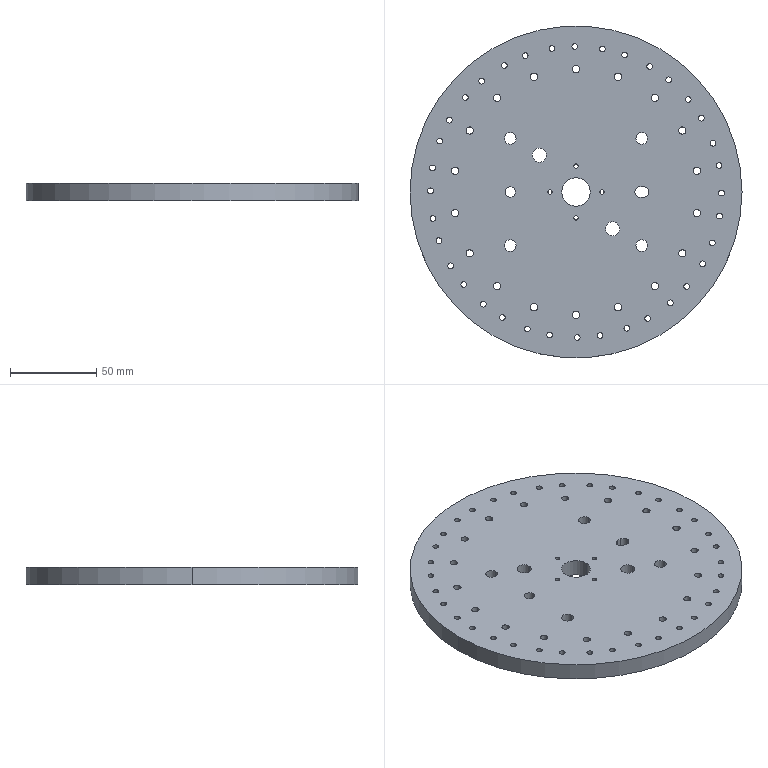Part | SolidWorks | features ICE 5, HoleWzd 3, 3DProfileFeature 2, CirPattern 2, Cut 2, Extrusion 1 | 1 solid | 141 faces | box 192 x 192 x 10 mm | volume 278427 mm3 | cylinder 137 | plane 4 | commonest cylinder face diameters 3.3 x72 4.2 x36 2.5 x8 6.8 x8 6 x5 8.2 x4